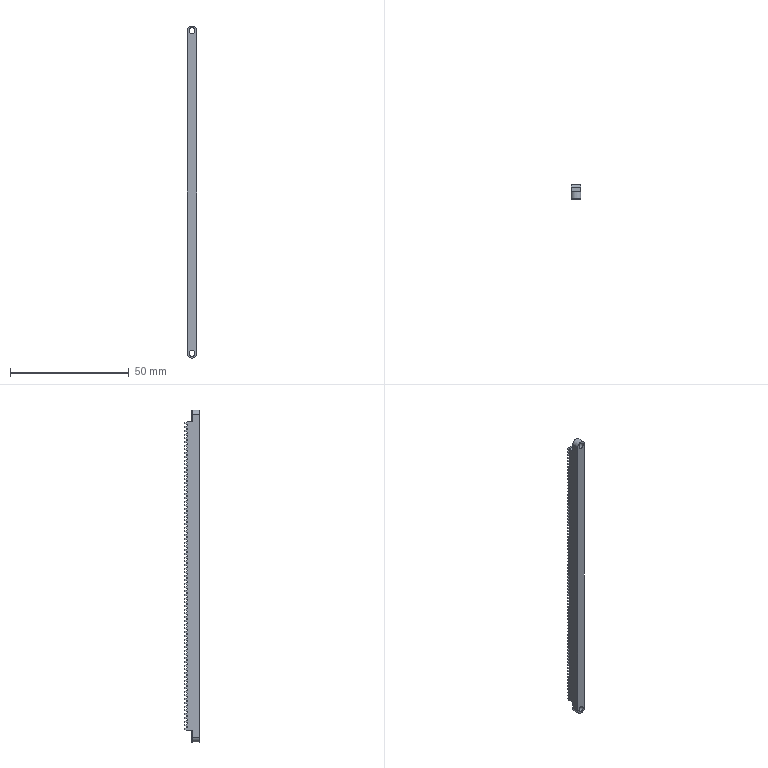Part | SolidWorks | features BaseBody 1 | 1 solid | 345 faces | box 4.026 x 6.017 x 140 mm | volume 2926 mm3 | plane 339 | cylinder 6 | commonest cylinder face diameters 2.5 x4 4 x2